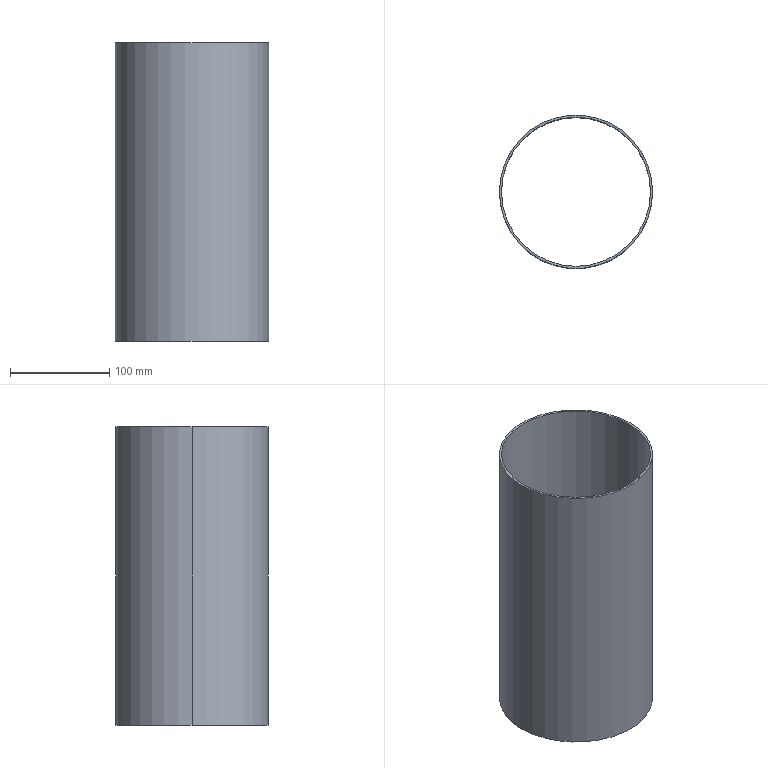Part | SolidWorks | features Extrusion 1 | 1 solid | 6 faces | box 154 x 154 x 300 mm | volume 286513 mm3 | cylinder 4 | plane 2 | commonest cylinder face diameters 150 x2 154 x2
STEP:
#1=CARTESIAN_POINT('',(-75.,0.,300.));
#2=VERTEX_POINT('',#1);
#3=CARTESIAN_POINT('',(75.,0.,300.));
#4=VERTEX_POINT('',#3);
#5=CARTESIAN_POINT('',(0.,0.,300.));
#6=DIRECTION('',(0.,0.,1.));
#7=DIRECTION('',(1.,0.,0.));
#8=AXIS2_PLACEMENT_3D('',#5,#6,#7);
#9=CIRCLE('',#8,75.);
#10=EDGE_CURVE('',#2,#4,#9,.T.);
#11=ORIENTED_EDGE('',*,*,#10,.T.);
#12=CARTESIAN_POINT('',(75.,0.,0.));
#13=VERTEX_POINT('',#12);
#14=CARTESIAN_POINT('',(75.,0.,300.));
#15=DIRECTION('',(0.,0.,-1.));
#16=VECTOR('',#15,1000.);
#17=LINE('',#14,#16);
#18=EDGE_CURVE('',#4,#13,#17,.T.);
#19=ORIENTED_EDGE('',*,*,#18,.T.);
#20=CARTESIAN_POINT('',(-75.,0.,0.));
#21=VERTEX_POINT('',#20);
#22=CARTESIAN_POINT('',(0.,0.,0.));
#23=DIRECTION('',(0.,0.,1.));
#24=DIRECTION('',(1.,0.,0.));
#25=AXIS2_PLACEMENT_3D('',#22,#23,#24);
#26=CIRCLE('',#25,75.);
#27=EDGE_CURVE('',#21,#13,#26,.T.);
#28=ORIENTED_EDGE('',*,*,#27,.F.);
#29=CARTESIAN_POINT('',(-75.,0.,300.));
#30=DIRECTION('',(0.,0.,-1.));
#31=VECTOR('',#30,1000.);
#32=LINE('',#29,#31);
#33=EDGE_CURVE('',#2,#21,#32,.T.);
#34=ORIENTED_EDGE('',*,*,#33,.F.);
#35=EDGE_LOOP('',(#11,#19,#28,#34));
#36=FACE_OUTER_BOUND('',#35,.T.);
#37=CARTESIAN_POINT('',(0.,0.,300.));
#38=DIRECTION('',(0.,0.,-1.));
#39=DIRECTION('',(-1.,0.,0.));
#40=AXIS2_PLACEMENT_3D('',#37,#38,#39);
#41=CYLINDRICAL_SURFACE('',#40,75.);
#42=ADVANCED_FACE('',(#36),#41,.F.);
#43=CARTESIAN_POINT('',(77.,0.,300.));
#44=VERTEX_POINT('',#43);
#45=CARTESIAN_POINT('',(-77.,0.,300.));
#46=VERTEX_POINT('',#45);
#47=CARTESIAN_POINT('',(0.,0.,300.));
#48=DIRECTION('',(0.,0.,1.));
#49=DIRECTION('',(1.,0.,0.));
#50=AXIS2_PLACEMENT_3D('',#47,#48,#49);
#51=CIRCLE('',#50,77.);
#52=EDGE_CURVE('',#44,#46,#51,.T.);
#53=ORIENTED_EDGE('',*,*,#52,.F.);
#54=CARTESIAN_POINT('',(77.,0.,0.));
#55=VERTEX_POINT('',#54);
#56=CARTESIAN_POINT('',(77.,0.,300.));
#57=DIRECTION('',(0.,0.,-1.));
#58=VECTOR('',#57,1000.);
#59=LINE('',#56,#58);
#60=EDGE_CURVE('',#44,#55,#59,.T.);
#61=ORIENTED_EDGE('',*,*,#60,.T.);
#62=CARTESIAN_POINT('',(-77.,0.,0.));
#63=VERTEX_POINT('',#62);
#64=CARTESIAN_POINT('',(0.,0.,0.));
#65=DIRECTION('',(0.,0.,1.));
#66=DIRECTION('',(1.,0.,0.));
#67=AXIS2_PLACEMENT_3D('',#64,#65,#66);
#68=CIRCLE('',#67,77.);
#69=EDGE_CURVE('',#55,#63,#68,.T.);
#70=ORIENTED_EDGE('',*,*,#69,.T.);
#71=CARTESIAN_POINT('',(-77.,0.,300.));
#72=DIRECTION('',(0.,0.,-1.));
#73=VECTOR('',#72,1000.);
#74=LINE('',#71,#73);
#75=EDGE_CURVE('',#46,#63,#74,.T.);
#76=ORIENTED_EDGE('',*,*,#75,.F.);
#77=EDGE_LOOP('',(#53,#61,#70,#76));
#78=FACE_OUTER_BOUND('',#77,.T.);
#79=CARTESIAN_POINT('',(0.,0.,300.));
#80=DIRECTION('',(0.,0.,-1.));
#81=DIRECTION('',(-1.,0.,0.));
#82=AXIS2_PLACEMENT_3D('',#79,#80,#81);
#83=CYLINDRICAL_SURFACE('',#82,77.);
#84=ADVANCED_FACE('',(#78),#83,.T.);
#85=CARTESIAN_POINT('',(0.,0.,300.));
#86=DIRECTION('',(0.,0.,1.));
#87=DIRECTION('',(1.,0.,0.));
#88=AXIS2_PLACEMENT_3D('',#85,#86,#87);
#89=CIRCLE('',#88,77.);
#90=EDGE_CURVE('',#46,#44,#89,.T.);
#91=ORIENTED_EDGE('',*,*,#90,.T.);
#92=ORIENTED_EDGE('',*,*,#52,.T.);
#93=EDGE_LOOP('',(#91,#92));
#94=FACE_OUTER_BOUND('',#93,.T.);
#95=ORIENTED_EDGE('',*,*,#10,.F.);
#96=CARTESIAN_POINT('',(0.,0.,300.));
#97=DIRECTION('',(0.,0.,1.));
#98=DIRECTION('',(1.,0.,0.));
#99=AXIS2_PLACEMENT_3D('',#96,#97,#98);
#100=CIRCLE('',#99,75.);
#101=EDGE_CURVE('',#4,#2,#100,.T.);
#102=ORIENTED_EDGE('',*,*,#101,.F.);
#103=EDGE_LOOP('',(#95,#102));
#104=FACE_BOUND('',#103,.T.);
#105=CARTESIAN_POINT('',(0.,0.,300.));
#106=DIRECTION('',(0.,0.,1.));
#107=DIRECTION('',(1.,0.,0.));
#108=AXIS2_PLACEMENT_3D('',#105,#106,#107);
#109=PLANE('',#108);
#110=ADVANCED_FACE('',(#94,#104),#109,.T.);
#111=CARTESIAN_POINT('',(0.,0.,0.));
#112=DIRECTION('',(0.,0.,1.));
#113=DIRECTION('',(1.,0.,0.));
#114=AXIS2_PLACEMENT_3D('',#111,#112,#113);
#115=CIRCLE('',#114,77.);
#116=EDGE_CURVE('',#63,#55,#115,.T.);
#117=ORIENTED_EDGE('',*,*,#116,.F.);
#118=ORIENTED_EDGE('',*,*,#69,.F.);
#119=EDGE_LOOP('',(#117,#118));
#120=FACE_OUTER_BOUND('',#119,.T.);
#121=ORIENTED_EDGE('',*,*,#27,.T.);
#122=CARTESIAN_POINT('',(0.,0.,0.));
#123=DIRECTION('',(0.,0.,1.));
#124=DIRECTION('',(1.,0.,0.));
#125=AXIS2_PLACEMENT_3D('',#122,#123,#124);
#126=CIRCLE('',#125,75.);
#127=EDGE_CURVE('',#13,#21,#126,.T.);
#128=ORIENTED_EDGE('',*,*,#127,.T.);
#129=EDGE_LOOP('',(#121,#128));
#130=FACE_BOUND('',#129,.T.);
#131=CARTESIAN_POINT('',(0.,0.,0.));
#132=DIRECTION('',(0.,0.,1.));
#133=DIRECTION('',(1.,0.,0.));
#134=AXIS2_PLACEMENT_3D('',#131,#132,#133);
#135=PLANE('',#134);
#136=ADVANCED_FACE('',(#120,#130),#135,.F.);
#137=ORIENTED_EDGE('',*,*,#60,.F.);
#138=ORIENTED_EDGE('',*,*,#90,.F.);
#139=ORIENTED_EDGE('',*,*,#75,.T.);
#140=ORIENTED_EDGE('',*,*,#116,.T.);
#141=EDGE_LOOP('',(#137,#138,#139,#140));
#142=FACE_OUTER_BOUND('',#141,.T.);
#143=CARTESIAN_POINT('',(0.,0.,300.));
#144=DIRECTION('',(0.,0.,-1.));
#145=DIRECTION('',(-1.,0.,0.));
#146=AXIS2_PLACEMENT_3D('',#143,#144,#145);
#147=CYLINDRICAL_SURFACE('',#146,77.);
#148=ADVANCED_FACE('',(#142),#147,.T.);
#149=ORIENTED_EDGE('',*,*,#18,.F.);
#150=ORIENTED_EDGE('',*,*,#101,.T.);
#151=ORIENTED_EDGE('',*,*,#33,.T.);
#152=ORIENTED_EDGE('',*,*,#127,.F.);
#153=EDGE_LOOP('',(#149,#150,#151,#152));
#154=FACE_OUTER_BOUND('',#153,.T.);
#155=CARTESIAN_POINT('',(0.,0.,300.));
#156=DIRECTION('',(0.,0.,-1.));
#157=DIRECTION('',(-1.,0.,0.));
#158=AXIS2_PLACEMENT_3D('',#155,#156,#157);
#159=CYLINDRICAL_SURFACE('',#158,75.);
#160=ADVANCED_FACE('',(#154),#159,.F.);
#161=CLOSED_SHELL('',(#42,#84,#110,#136,#148,#160));
#162=MANIFOLD_SOLID_BREP('',#161);
#163=CARTESIAN_POINT('',(0.,0.,0.));
#164=DIRECTION('',(0.,0.,1.));
#165=DIRECTION('',(1.,0.,0.));
#166=AXIS2_PLACEMENT_3D('',#163,#164,#165);
#167=(LENGTH_UNIT()NAMED_UNIT(*)SI_UNIT(.MILLI.,.METRE.));
#168=UNCERTAINTY_MEASURE_WITH_UNIT(LENGTH_MEASURE(0.00001),#167,'','');
#169=(NAMED_UNIT(*)PLANE_ANGLE_UNIT()SI_UNIT($,.RADIAN.));
#170=(NAMED_UNIT(*)SI_UNIT($,.STERADIAN.)SOLID_ANGLE_UNIT());
#171=(GEOMETRIC_REPRESENTATION_CONTEXT(3)GLOBAL_UNCERTAINTY_ASSIGNED_CONTEXT((#168))GLOBAL_UNIT_ASSIGNED_CONTEXT((#167,#169,#170))REPRESENTATION_CONTEXT('',''));
#172=ADVANCED_BREP_SHAPE_REPRESENTATION('',(#162,#166),#171);